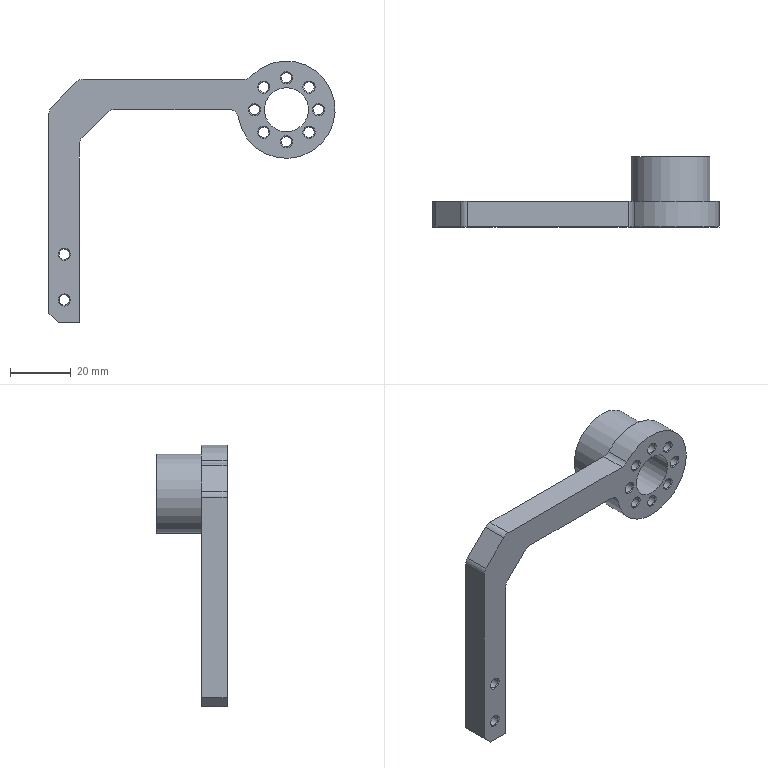Part | NX | features DATUM_CSYS 12, SKETCH 11, SIMPLE HOLE 10, HOLE PACKAGE 9, EXTRACT_FACE 8, Instance Feature 7, BLEND 2, CHAMFER 2, CPROJ 1, DATUM_AXIS 1, EXTRUDE 1, LINKED_FACE 1, OFFSET_REGION 1, Pattern Feature 1, SWP104 1 | 1 solid | 52 faces | box 93.991 x 23.1 x 85.991 mm | volume 19432 mm3 | cylinder 20 | cone 20 | plane 12 | commonest cylinder face diameters 3.4 x10 6 x6 14.463 x1 25.981 x1 29.983 x1 31.983 x1
STEP:
#1=CARTESIAN_POINT('',(-13.5,-14.1,-21.731));
#2=VERTEX_POINT('',#1);
#3=CARTESIAN_POINT('',(-13.5,-14.1,-14.5));
#4=DIRECTION('',(0.,-1.,0.));
#5=DIRECTION('',(0.,0.,-1.));
#6=AXIS2_PLACEMENT_3D('',#3,#4,#5);
#7=CIRCLE('',#6,7.231);
#8=EDGE_CURVE('',#2,#2,#7,.T.);
#9=ORIENTED_EDGE('',*,*,#8,.T.);
#10=EDGE_LOOP('',(#9));
#11=FACE_BOUND('',#10,.T.);
#12=CARTESIAN_POINT('',(-13.5,9.,-21.731));
#13=VERTEX_POINT('',#12);
#14=CARTESIAN_POINT('',(-13.5,9.,-14.5));
#15=DIRECTION('',(0.,-1.,0.));
#16=DIRECTION('',(0.,0.,-1.));
#17=AXIS2_PLACEMENT_3D('',#14,#15,#16);
#18=CIRCLE('',#17,7.231);
#19=EDGE_CURVE('',#13,#13,#18,.T.);
#20=ORIENTED_EDGE('',*,*,#19,.F.);
#21=EDGE_LOOP('',(#20));
#22=FACE_BOUND('',#21,.T.);
#23=CARTESIAN_POINT('',(-13.5,-13.36,-14.5));
#24=DIRECTION('',(0.,-1.,0.));
#25=DIRECTION('',(0.,0.,-1.));
#26=AXIS2_PLACEMENT_3D('',#23,#24,#25);
#27=CYLINDRICAL_SURFACE('',#26,7.231);
#28=ADVANCED_FACE('',(#11,#22),#27,.F.);
#29=CARTESIAN_POINT('',(-86.5,-14.1,-79.));
#30=VERTEX_POINT('',#29);
#31=CARTESIAN_POINT('',(-86.5,-14.1,-77.));
#32=DIRECTION('',(0.,-1.,0.));
#33=DIRECTION('',(0.,0.,-1.));
#34=AXIS2_PLACEMENT_3D('',#31,#32,#33);
#35=CIRCLE('',#34,2.);
#36=EDGE_CURVE('',#30,#30,#35,.F.);
#37=ORIENTED_EDGE('',*,*,#36,.T.);
#38=EDGE_LOOP('',(#37));
#39=FACE_BOUND('',#38,.T.);
#40=CARTESIAN_POINT('',(-86.5,-14.1,-64.));
#41=VERTEX_POINT('',#40);
#42=CARTESIAN_POINT('',(-86.5,-14.1,-62.));
#43=DIRECTION('',(0.,-1.,0.));
#44=DIRECTION('',(0.,0.,-1.));
#45=AXIS2_PLACEMENT_3D('',#42,#43,#44);
#46=CIRCLE('',#45,2.);
#47=EDGE_CURVE('',#41,#41,#46,.F.);
#48=ORIENTED_EDGE('',*,*,#47,.T.);
#49=EDGE_LOOP('',(#48));
#50=FACE_BOUND('',#49,.T.);
#51=CARTESIAN_POINT('',(-6.075,-14.1,-9.075));
#52=VERTEX_POINT('',#51);
#53=CARTESIAN_POINT('',(-6.075,-14.1,-7.075));
#54=DIRECTION('',(0.,-1.,0.));
#55=DIRECTION('',(0.,0.,-1.));
#56=AXIS2_PLACEMENT_3D('',#53,#54,#55);
#57=CIRCLE('',#56,2.);
#58=EDGE_CURVE('',#52,#52,#57,.F.);
#59=ORIENTED_EDGE('',*,*,#58,.T.);
#60=EDGE_LOOP('',(#59));
#61=FACE_BOUND('',#60,.T.);
#62=CARTESIAN_POINT('',(-3.,-14.1,-16.5));
#63=VERTEX_POINT('',#62);
#64=CARTESIAN_POINT('',(-3.,-14.1,-14.5));
#65=DIRECTION('',(0.,-1.,0.));
#66=DIRECTION('',(0.,0.,-1.));
#67=AXIS2_PLACEMENT_3D('',#64,#65,#66);
#68=CIRCLE('',#67,2.);
#69=EDGE_CURVE('',#63,#63,#68,.F.);
#70=ORIENTED_EDGE('',*,*,#69,.T.);
#71=EDGE_LOOP('',(#70));
#72=FACE_BOUND('',#71,.T.);
#73=CARTESIAN_POINT('',(-6.075,-14.1,-23.925));
#74=VERTEX_POINT('',#73);
#75=CARTESIAN_POINT('',(-6.075,-14.1,-21.925));
#76=DIRECTION('',(0.,-1.,0.));
#77=DIRECTION('',(0.,0.,-1.));
#78=AXIS2_PLACEMENT_3D('',#75,#76,#77);
#79=CIRCLE('',#78,2.);
#80=EDGE_CURVE('',#74,#74,#79,.F.);
#81=ORIENTED_EDGE('',*,*,#80,.T.);
#82=EDGE_LOOP('',(#81));
#83=FACE_BOUND('',#82,.T.);
#84=CARTESIAN_POINT('',(-13.5,-14.1,-27.));
#85=VERTEX_POINT('',#84);
#86=CARTESIAN_POINT('',(-13.5,-14.1,-25.));
#87=DIRECTION('',(0.,-1.,0.));
#88=DIRECTION('',(0.,0.,-1.));
#89=AXIS2_PLACEMENT_3D('',#86,#87,#88);
#90=CIRCLE('',#89,2.);
#91=EDGE_CURVE('',#85,#85,#90,.F.);
#92=ORIENTED_EDGE('',*,*,#91,.T.);
#93=EDGE_LOOP('',(#92));
#94=FACE_BOUND('',#93,.T.);
#95=CARTESIAN_POINT('',(-20.925,-14.1,-23.925));
#96=VERTEX_POINT('',#95);
#97=CARTESIAN_POINT('',(-20.925,-14.1,-21.925));
#98=DIRECTION('',(0.,-1.,0.));
#99=DIRECTION('',(0.,0.,-1.));
#100=AXIS2_PLACEMENT_3D('',#97,#98,#99);
#101=CIRCLE('',#100,2.);
#102=EDGE_CURVE('',#96,#96,#101,.F.);
#103=ORIENTED_EDGE('',*,*,#102,.T.);
#104=EDGE_LOOP('',(#103));
#105=FACE_BOUND('',#104,.T.);
#106=CARTESIAN_POINT('',(-24.,-14.1,-16.5));
#107=VERTEX_POINT('',#106);
#108=CARTESIAN_POINT('',(-24.,-14.1,-14.5));
#109=DIRECTION('',(0.,-1.,0.));
#110=DIRECTION('',(0.,0.,-1.));
#111=AXIS2_PLACEMENT_3D('',#108,#109,#110);
#112=CIRCLE('',#111,2.);
#113=EDGE_CURVE('',#107,#107,#112,.F.);
#114=ORIENTED_EDGE('',*,*,#113,.T.);
#115=EDGE_LOOP('',(#114));
#116=FACE_BOUND('',#115,.T.);
#117=CARTESIAN_POINT('',(-20.925,-14.1,-9.075));
#118=VERTEX_POINT('',#117);
#119=CARTESIAN_POINT('',(-20.925,-14.1,-7.075));
#120=DIRECTION('',(0.,-1.,0.));
#121=DIRECTION('',(0.,0.,-1.));
#122=AXIS2_PLACEMENT_3D('',#119,#120,#121);
#123=CIRCLE('',#122,2.);
#124=EDGE_CURVE('',#118,#118,#123,.F.);
#125=ORIENTED_EDGE('',*,*,#124,.T.);
#126=EDGE_LOOP('',(#125));
#127=FACE_BOUND('',#126,.T.);
#128=CARTESIAN_POINT('',(-13.5,-14.1,-6.));
#129=VERTEX_POINT('',#128);
#130=CARTESIAN_POINT('',(-13.5,-14.1,-4.));
#131=DIRECTION('',(0.,-1.,0.));
#132=DIRECTION('',(0.,0.,-1.));
#133=AXIS2_PLACEMENT_3D('',#130,#131,#132);
#134=CIRCLE('',#133,2.);
#135=EDGE_CURVE('',#129,#129,#134,.F.);
#136=ORIENTED_EDGE('',*,*,#135,.T.);
#137=EDGE_LOOP('',(#136));
#138=FACE_BOUND('',#137,.T.);
#139=CARTESIAN_POINT('',(-91.5,-14.1,-15.743));
#140=VERTEX_POINT('',#139);
#141=CARTESIAN_POINT('',(-91.5,-14.1,-81.5));
#142=VERTEX_POINT('',#141);
#143=CARTESIAN_POINT('',(-91.5,-14.1,-4.5));
#144=DIRECTION('',(0.,0.,-1.));
#145=VECTOR('',#144,1000.);
#146=LINE('',#143,#145);
#147=EDGE_CURVE('',#140,#142,#146,.T.);
#148=ORIENTED_EDGE('',*,*,#147,.T.);
#149=CARTESIAN_POINT('',(-88.5,-14.1,-84.5));
#150=VERTEX_POINT('',#149);
#151=CARTESIAN_POINT('',(-82.384,-14.1,-90.616));
#152=DIRECTION('',(-0.7071,0.,0.7071));
#153=VECTOR('',#152,1000.);
#154=LINE('',#151,#153);
#155=EDGE_CURVE('',#142,#150,#154,.F.);
#156=ORIENTED_EDGE('',*,*,#155,.T.);
#157=CARTESIAN_POINT('',(-81.5,-14.1,-84.5));
#158=VERTEX_POINT('',#157);
#159=CARTESIAN_POINT('',(-91.5,-14.1,-84.5));
#160=DIRECTION('',(1.,0.,0.));
#161=VECTOR('',#160,1000.);
#162=LINE('',#159,#161);
#163=EDGE_CURVE('',#150,#158,#162,.T.);
#164=ORIENTED_EDGE('',*,*,#163,.T.);
#165=CARTESIAN_POINT('',(-81.5,-14.1,-25.743));
#166=VERTEX_POINT('',#165);
#167=CARTESIAN_POINT('',(-81.5,-14.1,-84.5));
#168=DIRECTION('',(0.,0.,1.));
#169=VECTOR('',#168,1000.);
#170=LINE('',#167,#169);
#171=EDGE_CURVE('',#158,#166,#170,.T.);
#172=ORIENTED_EDGE('',*,*,#171,.T.);
#173=CARTESIAN_POINT('',(-80.621,-14.1,-23.621));
#174=VERTEX_POINT('',#173);
#175=CARTESIAN_POINT('',(-78.5,-14.1,-25.743));
#176=DIRECTION('',(0.,-1.,0.));
#177=DIRECTION('',(0.,0.,-1.));
#178=AXIS2_PLACEMENT_3D('',#175,#176,#177);
#179=CIRCLE('',#178,3.);
#180=EDGE_CURVE('',#166,#174,#179,.F.);
#181=ORIENTED_EDGE('',*,*,#180,.T.);
#182=CARTESIAN_POINT('',(-72.379,-14.1,-15.379));
#183=VERTEX_POINT('',#182);
#184=CARTESIAN_POINT('',(-81.5,-14.1,-24.5));
#185=DIRECTION('',(-0.7071,0.,-0.7071));
#186=VECTOR('',#185,1000.);
#187=LINE('',#184,#186);
#188=EDGE_CURVE('',#174,#183,#187,.F.);
#189=ORIENTED_EDGE('',*,*,#188,.T.);
#190=CARTESIAN_POINT('',(-70.257,-14.1,-14.5));
#191=VERTEX_POINT('',#190);
#192=CARTESIAN_POINT('',(-70.257,-14.1,-17.5));
#193=DIRECTION('',(0.,-1.,0.));
#194=DIRECTION('',(0.,0.,-1.));
#195=AXIS2_PLACEMENT_3D('',#192,#193,#194);
#196=CIRCLE('',#195,3.);
#197=EDGE_CURVE('',#183,#191,#196,.F.);
#198=ORIENTED_EDGE('',*,*,#197,.T.);
#199=CARTESIAN_POINT('',(-32.253,-14.1,-14.5));
#200=VERTEX_POINT('',#199);
#201=CARTESIAN_POINT('',(-81.5,-14.1,-14.5));
#202=DIRECTION('',(1.,0.,0.));
#203=VECTOR('',#202,1000.);
#204=LINE('',#201,#203);
#205=EDGE_CURVE('',#191,#200,#204,.T.);
#206=ORIENTED_EDGE('',*,*,#205,.T.);
#207=CARTESIAN_POINT('',(-29.291,-14.1,-17.026));
#208=VERTEX_POINT('',#207);
#209=CARTESIAN_POINT('',(-32.253,-14.1,-17.5));
#210=DIRECTION('',(0.,-1.,0.));
#211=DIRECTION('',(0.,0.,-1.));
#212=AXIS2_PLACEMENT_3D('',#209,#210,#211);
#213=CIRCLE('',#212,3.);
#214=EDGE_CURVE('',#200,#208,#213,.F.);
#215=ORIENTED_EDGE('',*,*,#214,.T.);
#216=CARTESIAN_POINT('',(-25.158,-14.1,-3.554));
#217=VERTEX_POINT('',#216);
#218=CARTESIAN_POINT('',(-13.5,-14.1,-14.5));
#219=DIRECTION('',(0.,-1.,0.));
#220=DIRECTION('',(0.,0.,-1.));
#221=AXIS2_PLACEMENT_3D('',#218,#219,#220);
#222=CIRCLE('',#221,15.991);
#223=EDGE_CURVE('',#208,#217,#222,.T.);
#224=ORIENTED_EDGE('',*,*,#223,.T.);
#225=CARTESIAN_POINT('',(-27.345,-14.1,-4.5));
#226=VERTEX_POINT('',#225);
#227=CARTESIAN_POINT('',(-27.345,-14.1,-1.5));
#228=DIRECTION('',(0.,-1.,0.));
#229=DIRECTION('',(0.,0.,-1.));
#230=AXIS2_PLACEMENT_3D('',#227,#228,#229);
#231=CIRCLE('',#230,3.);
#232=EDGE_CURVE('',#217,#226,#231,.F.);
#233=ORIENTED_EDGE('',*,*,#232,.T.);
#234=CARTESIAN_POINT('',(-80.257,-14.1,-4.5));
#235=VERTEX_POINT('',#234);
#236=CARTESIAN_POINT('',(-81.5,-14.1,-4.5));
#237=DIRECTION('',(-1.,0.,0.));
#238=VECTOR('',#237,1000.);
#239=LINE('',#236,#238);
#240=EDGE_CURVE('',#226,#235,#239,.T.);
#241=ORIENTED_EDGE('',*,*,#240,.T.);
#242=CARTESIAN_POINT('',(-82.379,-14.1,-5.379));
#243=VERTEX_POINT('',#242);
#244=CARTESIAN_POINT('',(-80.257,-14.1,-7.5));
#245=DIRECTION('',(0.,-1.,0.));
#246=DIRECTION('',(0.,0.,-1.));
#247=AXIS2_PLACEMENT_3D('',#244,#245,#246);
#248=CIRCLE('',#247,3.);
#249=EDGE_CURVE('',#235,#243,#248,.T.);
#250=ORIENTED_EDGE('',*,*,#249,.T.);
#251=CARTESIAN_POINT('',(-90.621,-14.1,-13.621));
#252=VERTEX_POINT('',#251);
#253=CARTESIAN_POINT('',(-48.884,-14.1,28.116));
#254=DIRECTION('',(0.7071,0.,0.7071));
#255=VECTOR('',#254,1000.);
#256=LINE('',#253,#255);
#257=EDGE_CURVE('',#243,#252,#256,.F.);
#258=ORIENTED_EDGE('',*,*,#257,.T.);
#259=CARTESIAN_POINT('',(-88.5,-14.1,-15.743));
#260=DIRECTION('',(0.,-1.,0.));
#261=DIRECTION('',(0.,0.,-1.));
#262=AXIS2_PLACEMENT_3D('',#259,#260,#261);
#263=CIRCLE('',#262,3.);
#264=EDGE_CURVE('',#252,#140,#263,.T.);
#265=ORIENTED_EDGE('',*,*,#264,.T.);
#266=EDGE_LOOP('',(#148,#156,#164,#172,#181,#189,#198,#206,#215,#224,#233,#241,#250,#258,#265));
#267=FACE_BOUND('',#266,.T.);
#268=ORIENTED_EDGE('',*,*,#8,.F.);
#269=EDGE_LOOP('',(#268));
#270=FACE_BOUND('',#269,.T.);
#271=CARTESIAN_POINT('',(-6.269,-14.1,-14.5));
#272=DIRECTION('',(0.,-1.,0.));
#273=DIRECTION('',(0.,0.,-1.));
#274=AXIS2_PLACEMENT_3D('',#271,#272,#273);
#275=PLANE('',#274);
#276=ADVANCED_FACE('',(#39,#50,#61,#72,#83,#94,#105,#116,#127,#138,#267,#270),#275,.T.);
#277=ORIENTED_EDGE('',*,*,#223,.F.);
#278=CARTESIAN_POINT('',(-29.291,-5.6,-17.026));
#279=VERTEX_POINT('',#278);
#280=CARTESIAN_POINT('',(-29.291,-13.36,-17.026));
#281=DIRECTION('',(0.,-1.,0.));
#282=VECTOR('',#281,1000.);
#283=LINE('',#280,#282);
#284=EDGE_CURVE('',#208,#279,#283,.F.);
#285=ORIENTED_EDGE('',*,*,#284,.T.);
#286=CARTESIAN_POINT('',(-25.158,-5.6,-3.554));
#287=VERTEX_POINT('',#286);
#288=CARTESIAN_POINT('',(-13.5,-5.6,-14.5));
#289=DIRECTION('',(0.,-1.,0.));
#290=DIRECTION('',(0.,0.,-1.));
#291=AXIS2_PLACEMENT_3D('',#288,#289,#290);
#292=CIRCLE('',#291,15.991);
#293=EDGE_CURVE('',#279,#287,#292,.T.);
#294=ORIENTED_EDGE('',*,*,#293,.T.);
#295=CARTESIAN_POINT('',(-25.158,-13.36,-3.554));
#296=DIRECTION('',(0.,-1.,0.));
#297=VECTOR('',#296,1000.);
#298=LINE('',#295,#297);
#299=EDGE_CURVE('',#287,#217,#298,.T.);
#300=ORIENTED_EDGE('',*,*,#299,.T.);
#301=EDGE_LOOP('',(#277,#285,#294,#300));
#302=FACE_BOUND('',#301,.T.);
#303=CARTESIAN_POINT('',(-13.5,-13.36,-14.5));
#304=DIRECTION('',(0.,-1.,0.));
#305=DIRECTION('',(0.,0.,-1.));
#306=AXIS2_PLACEMENT_3D('',#303,#304,#305);
#307=CYLINDRICAL_SURFACE('',#306,15.991);
#308=ADVANCED_FACE('',(#302),#307,.T.);
#309=CARTESIAN_POINT('',(-86.5,-5.6,-75.));
#310=VERTEX_POINT('',#309);
#311=CARTESIAN_POINT('',(-86.5,-5.6,-77.));
#312=DIRECTION('',(0.,1.,0.));
#313=DIRECTION('',(0.,0.,1.));
#314=AXIS2_PLACEMENT_3D('',#311,#312,#313);
#315=CIRCLE('',#314,2.);
#316=EDGE_CURVE('',#310,#310,#315,.F.);
#317=ORIENTED_EDGE('',*,*,#316,.T.);
#318=EDGE_LOOP('',(#317));
#319=FACE_BOUND('',#318,.T.);
#320=CARTESIAN_POINT('',(-86.5,-5.6,-60.));
#321=VERTEX_POINT('',#320);
#322=CARTESIAN_POINT('',(-86.5,-5.6,-62.));
#323=DIRECTION('',(0.,1.,0.));
#324=DIRECTION('',(0.,0.,1.));
#325=AXIS2_PLACEMENT_3D('',#322,#323,#324);
#326=CIRCLE('',#325,2.);
#327=EDGE_CURVE('',#321,#321,#326,.F.);
#328=ORIENTED_EDGE('',*,*,#327,.T.);
#329=EDGE_LOOP('',(#328));
#330=FACE_BOUND('',#329,.T.);
#331=CARTESIAN_POINT('',(-13.5,-5.6,-29.491));
#332=VERTEX_POINT('',#331);
#333=CARTESIAN_POINT('',(-13.5,-5.6,-14.5));
#334=DIRECTION('',(0.,-1.,0.));
#335=DIRECTION('',(0.,0.,-1.));
#336=AXIS2_PLACEMENT_3D('',#333,#334,#335);
#337=CIRCLE('',#336,14.991);
#338=EDGE_CURVE('',#332,#332,#337,.T.);
#339=ORIENTED_EDGE('',*,*,#338,.T.);
#340=EDGE_LOOP('',(#339));
#341=FACE_BOUND('',#340,.T.);
#342=CARTESIAN_POINT('',(-88.5,-5.6,-84.5));
#343=VERTEX_POINT('',#342);
#344=CARTESIAN_POINT('',(-81.5,-5.6,-84.5));
#345=VERTEX_POINT('',#344);
#346=CARTESIAN_POINT('',(-91.5,-5.6,-84.5));
#347=DIRECTION('',(1.,0.,0.));
#348=VECTOR('',#347,1000.);
#349=LINE('',#346,#348);
#350=EDGE_CURVE('',#343,#345,#349,.T.);
#351=ORIENTED_EDGE('',*,*,#350,.F.);
#352=CARTESIAN_POINT('',(-91.5,-5.6,-81.5));
#353=VERTEX_POINT('',#352);
#354=CARTESIAN_POINT('',(-78.004,-5.6,-94.996));
#355=DIRECTION('',(0.7071,0.,-0.7071));
#356=VECTOR('',#355,1000.);
#357=LINE('',#354,#356);
#358=EDGE_CURVE('',#343,#353,#357,.F.);
#359=ORIENTED_EDGE('',*,*,#358,.T.);
#360=CARTESIAN_POINT('',(-91.5,-5.6,-15.743));
#361=VERTEX_POINT('',#360);
#362=CARTESIAN_POINT('',(-91.5,-5.6,-14.5));
#363=DIRECTION('',(0.,0.,-1.));
#364=VECTOR('',#363,1000.);
#365=LINE('',#362,#364);
#366=EDGE_CURVE('',#361,#353,#365,.T.);
#367=ORIENTED_EDGE('',*,*,#366,.F.);
#368=CARTESIAN_POINT('',(-90.621,-5.6,-13.621));
#369=VERTEX_POINT('',#368);
#370=CARTESIAN_POINT('',(-88.5,-5.6,-15.743));
#371=DIRECTION('',(0.,1.,0.));
#372=DIRECTION('',(0.,0.,1.));
#373=AXIS2_PLACEMENT_3D('',#370,#371,#372);
#374=CIRCLE('',#373,3.);
#375=EDGE_CURVE('',#361,#369,#374,.T.);
#376=ORIENTED_EDGE('',*,*,#375,.T.);
#377=CARTESIAN_POINT('',(-82.379,-5.6,-5.379));
#378=VERTEX_POINT('',#377);
#379=CARTESIAN_POINT('',(-44.504,-5.6,32.496));
#380=DIRECTION('',(-0.7071,0.,-0.7071));
#381=VECTOR('',#380,1000.);
#382=LINE('',#379,#381);
#383=EDGE_CURVE('',#369,#378,#382,.F.);
#384=ORIENTED_EDGE('',*,*,#383,.T.);
#385=CARTESIAN_POINT('',(-80.257,-5.6,-4.5));
#386=VERTEX_POINT('',#385);
#387=CARTESIAN_POINT('',(-80.257,-5.6,-7.5));
#388=DIRECTION('',(0.,1.,0.));
#389=DIRECTION('',(0.,0.,1.));
#390=AXIS2_PLACEMENT_3D('',#387,#388,#389);
#391=CIRCLE('',#390,3.);
#392=EDGE_CURVE('',#378,#386,#391,.T.);
#393=ORIENTED_EDGE('',*,*,#392,.T.);
#394=CARTESIAN_POINT('',(-27.345,-5.6,-4.5));
#395=VERTEX_POINT('',#394);
#396=CARTESIAN_POINT('',(-25.979,-5.6,-4.5));
#397=DIRECTION('',(-1.,0.,0.));
#398=VECTOR('',#397,1000.);
#399=LINE('',#396,#398);
#400=EDGE_CURVE('',#395,#386,#399,.T.);
#401=ORIENTED_EDGE('',*,*,#400,.F.);
#402=CARTESIAN_POINT('',(-27.345,-5.6,-1.5));
#403=DIRECTION('',(0.,1.,0.));
#404=DIRECTION('',(0.,0.,1.));
#405=AXIS2_PLACEMENT_3D('',#402,#403,#404);
#406=CIRCLE('',#405,3.);
#407=EDGE_CURVE('',#395,#287,#406,.F.);
#408=ORIENTED_EDGE('',*,*,#407,.T.);
#409=ORIENTED_EDGE('',*,*,#293,.F.);
#410=CARTESIAN_POINT('',(-32.253,-5.6,-14.5));
#411=VERTEX_POINT('',#410);
#412=CARTESIAN_POINT('',(-32.253,-5.6,-17.5));
#413=DIRECTION('',(0.,1.,0.));
#414=DIRECTION('',(0.,0.,1.));
#415=AXIS2_PLACEMENT_3D('',#412,#413,#414);
#416=CIRCLE('',#415,3.);
#417=EDGE_CURVE('',#279,#411,#416,.F.);
#418=ORIENTED_EDGE('',*,*,#417,.T.);
#419=CARTESIAN_POINT('',(-70.257,-5.6,-14.5));
#420=VERTEX_POINT('',#419);
#421=CARTESIAN_POINT('',(-81.5,-5.6,-14.5));
#422=DIRECTION('',(1.,0.,0.));
#423=VECTOR('',#422,1000.);
#424=LINE('',#421,#423);
#425=EDGE_CURVE('',#420,#411,#424,.T.);
#426=ORIENTED_EDGE('',*,*,#425,.F.);
#427=CARTESIAN_POINT('',(-72.379,-5.6,-15.379));
#428=VERTEX_POINT('',#427);
#429=CARTESIAN_POINT('',(-70.257,-5.6,-17.5));
#430=DIRECTION('',(0.,1.,0.));
#431=DIRECTION('',(0.,0.,1.));
#432=AXIS2_PLACEMENT_3D('',#429,#430,#431);
#433=CIRCLE('',#432,3.);
#434=EDGE_CURVE('',#420,#428,#433,.F.);
#435=ORIENTED_EDGE('',*,*,#434,.T.);
#436=CARTESIAN_POINT('',(-80.621,-5.6,-23.621));
#437=VERTEX_POINT('',#436);
#438=CARTESIAN_POINT('',(-81.5,-5.6,-24.5));
#439=DIRECTION('',(0.7071,0.,0.7071));
#440=VECTOR('',#439,1000.);
#441=LINE('',#438,#440);
#442=EDGE_CURVE('',#428,#437,#441,.F.);
#443=ORIENTED_EDGE('',*,*,#442,.T.);
#444=CARTESIAN_POINT('',(-81.5,-5.6,-25.743));
#445=VERTEX_POINT('',#444);
#446=CARTESIAN_POINT('',(-78.5,-5.6,-25.743));
#447=DIRECTION('',(0.,1.,0.));
#448=DIRECTION('',(0.,0.,1.));
#449=AXIS2_PLACEMENT_3D('',#446,#447,#448);
#450=CIRCLE('',#449,3.);
#451=EDGE_CURVE('',#437,#445,#450,.F.);
#452=ORIENTED_EDGE('',*,*,#451,.T.);
#453=CARTESIAN_POINT('',(-81.5,-5.6,-84.5));
#454=DIRECTION('',(0.,0.,1.));
#455=VECTOR('',#454,1000.);
#456=LINE('',#453,#455);
#457=EDGE_CURVE('',#345,#445,#456,.T.);
#458=ORIENTED_EDGE('',*,*,#457,.F.);
#459=EDGE_LOOP('',(#351,#359,#367,#376,#384,#393,#401,#408,#409,#418,#426,#435,#443,#452,#458));
#460=FACE_BOUND('',#459,.T.);
#461=CARTESIAN_POINT('',(2.491,-5.6,-14.5));
#462=DIRECTION('',(0.,1.,0.));
#463=DIRECTION('',(0.,0.,1.));
#464=AXIS2_PLACEMENT_3D('',#461,#462,#463);
#465=PLANE('',#464);
#466=ADVANCED_FACE('',(#319,#330,#341,#460),#465,.T.);
#467=CARTESIAN_POINT('',(-13.5,-10.1,0.4914));
#468=VERTEX_POINT('',#467);
#469=CARTESIAN_POINT('',(-13.5,-10.1,-14.5));
#470=DIRECTION('',(0.,1.,0.));
#471=DIRECTION('',(0.,0.,1.));
#472=AXIS2_PLACEMENT_3D('',#469,#470,#471);
#473=CIRCLE('',#472,14.991);
#474=EDGE_CURVE('',#468,#468,#473,.F.);
#475=ORIENTED_EDGE('',*,*,#474,.T.);
#476=EDGE_LOOP('',(#475));
#477=FACE_BOUND('',#476,.T.);
#478=ORIENTED_EDGE('',*,*,#338,.F.);
#479=EDGE_LOOP('',(#478));
#480=FACE_BOUND('',#479,.T.);
#481=CARTESIAN_POINT('',(-13.5,-13.36,-14.5));
#482=DIRECTION('',(0.,-1.,0.));
#483=DIRECTION('',(0.,0.,-1.));
#484=AXIS2_PLACEMENT_3D('',#481,#482,#483);
#485=CYLINDRICAL_SURFACE('',#484,14.991);
#486=ADVANCED_FACE('',(#477,#480),#485,.F.);
#487=CARTESIAN_POINT('',(-13.5,-10.1,-1.509));
#488=VERTEX_POINT('',#487);
#489=CARTESIAN_POINT('',(-13.5,-10.1,-14.5));
#490=DIRECTION('',(0.,1.,0.));
#491=DIRECTION('',(0.,0.,1.));
#492=AXIS2_PLACEMENT_3D('',#489,#490,#491);
#493=CIRCLE('',#492,12.991);
#494=EDGE_CURVE('',#488,#488,#493,.F.);
#495=ORIENTED_EDGE('',*,*,#494,.T.);
#496=EDGE_LOOP('',(#495));
#497=FACE_BOUND('',#496,.T.);
#498=ORIENTED_EDGE('',*,*,#474,.F.);
#499=EDGE_LOOP('',(#498));
#500=FACE_BOUND('',#499,.T.);
#501=CARTESIAN_POINT('',(1.491,-10.1,-14.5));
#502=DIRECTION('',(0.,1.,0.));
#503=DIRECTION('',(0.,0.,1.));
#504=AXIS2_PLACEMENT_3D('',#501,#502,#503);
#505=PLANE('',#504);
#506=ADVANCED_FACE('',(#497,#500),#505,.T.);
#507=CARTESIAN_POINT('',(-13.5,9.,-27.491));
#508=VERTEX_POINT('',#507);
#509=CARTESIAN_POINT('',(-13.5,9.,-14.5));
#510=DIRECTION('',(0.,-1.,0.));
#511=DIRECTION('',(0.,0.,-1.));
#512=AXIS2_PLACEMENT_3D('',#509,#510,#511);
#513=CIRCLE('',#512,12.991);
#514=EDGE_CURVE('',#508,#508,#513,.T.);
#515=ORIENTED_EDGE('',*,*,#514,.T.);
#516=EDGE_LOOP('',(#515));
#517=FACE_BOUND('',#516,.T.);
#518=ORIENTED_EDGE('',*,*,#494,.F.);
#519=EDGE_LOOP('',(#518));
#520=FACE_BOUND('',#519,.T.);
#521=CARTESIAN_POINT('',(-13.5,-13.36,-14.5));
#522=DIRECTION('',(0.,-1.,0.));
#523=DIRECTION('',(0.,0.,-1.));
#524=AXIS2_PLACEMENT_3D('',#521,#522,#523);
#525=CYLINDRICAL_SURFACE('',#524,12.991);
#526=ADVANCED_FACE('',(#517,#520),#525,.T.);
#527=CARTESIAN_POINT('',(-6.075,9.,-5.075));
#528=VERTEX_POINT('',#527);
#529=CARTESIAN_POINT('',(-6.075,9.,-7.075));
#530=DIRECTION('',(0.,1.,0.));
#531=DIRECTION('',(0.,0.,1.));
#532=AXIS2_PLACEMENT_3D('',#529,#530,#531);
#533=CIRCLE('',#532,2.);
#534=EDGE_CURVE('',#528,#528,#533,.F.);
#535=ORIENTED_EDGE('',*,*,#534,.T.);
#536=EDGE_LOOP('',(#535));
#537=FACE_BOUND('',#536,.T.);
#538=CARTESIAN_POINT('',(-3.,9.,-12.5));
#539=VERTEX_POINT('',#538);
#540=CARTESIAN_POINT('',(-3.,9.,-14.5));
#541=DIRECTION('',(0.,1.,0.));
#542=DIRECTION('',(0.,0.,1.));
#543=AXIS2_PLACEMENT_3D('',#540,#541,#542);
#544=CIRCLE('',#543,2.);
#545=EDGE_CURVE('',#539,#539,#544,.F.);
#546=ORIENTED_EDGE('',*,*,#545,.T.);
#547=EDGE_LOOP('',(#546));
#548=FACE_BOUND('',#547,.T.);
#549=CARTESIAN_POINT('',(-6.075,9.,-19.925));
#550=VERTEX_POINT('',#549);
#551=CARTESIAN_POINT('',(-6.075,9.,-21.925));
#552=DIRECTION('',(0.,1.,0.));
#553=DIRECTION('',(0.,0.,1.));
#554=AXIS2_PLACEMENT_3D('',#551,#552,#553);
#555=CIRCLE('',#554,2.);
#556=EDGE_CURVE('',#550,#550,#555,.F.);
#557=ORIENTED_EDGE('',*,*,#556,.T.);
#558=EDGE_LOOP('',(#557));
#559=FACE_BOUND('',#558,.T.);
#560=CARTESIAN_POINT('',(-13.5,9.,-23.));
#561=VERTEX_POINT('',#560);
#562=CARTESIAN_POINT('',(-13.5,9.,-25.));
#563=DIRECTION('',(0.,1.,0.));
#564=DIRECTION('',(0.,0.,1.));
#565=AXIS2_PLACEMENT_3D('',#562,#563,#564);
#566=CIRCLE('',#565,2.);
#567=EDGE_CURVE('',#561,#561,#566,.F.);
#568=ORIENTED_EDGE('',*,*,#567,.T.);
#569=EDGE_LOOP('',(#568));
#570=FACE_BOUND('',#569,.T.);
#571=CARTESIAN_POINT('',(-20.925,9.,-19.925));
#572=VERTEX_POINT('',#571);
#573=CARTESIAN_POINT('',(-20.925,9.,-21.925));
#574=DIRECTION('',(0.,1.,0.));
#575=DIRECTION('',(0.,0.,1.));
#576=AXIS2_PLACEMENT_3D('',#573,#574,#575);
#577=CIRCLE('',#576,2.);
#578=EDGE_CURVE('',#572,#572,#577,.F.);
#579=ORIENTED_EDGE('',*,*,#578,.T.);
#580=EDGE_LOOP('',(#579));
#581=FACE_BOUND('',#580,.T.);
#582=CARTESIAN_POINT('',(-24.,9.,-12.5));
#583=VERTEX_POINT('',#582);
#584=CARTESIAN_POINT('',(-24.,9.,-14.5));
#585=DIRECTION('',(0.,1.,0.));
#586=DIRECTION('',(0.,0.,1.));
#587=AXIS2_PLACEMENT_3D('',#584,#585,#586);
#588=CIRCLE('',#587,2.);
#589=EDGE_CURVE('',#583,#583,#588,.F.);
#590=ORIENTED_EDGE('',*,*,#589,.T.);
#591=EDGE_LOOP('',(#590));
#592=FACE_BOUND('',#591,.T.);
#593=CARTESIAN_POINT('',(-20.925,9.,-5.075));
#594=VERTEX_POINT('',#593);
#595=CARTESIAN_POINT('',(-20.925,9.,-7.075));
#596=DIRECTION('',(0.,1.,0.));
#597=DIRECTION('',(0.,0.,1.));
#598=AXIS2_PLACEMENT_3D('',#595,#596,#597);
#599=CIRCLE('',#598,2.);
#600=EDGE_CURVE('',#594,#594,#599,.F.);
#601=ORIENTED_EDGE('',*,*,#600,.T.);
#602=EDGE_LOOP('',(#601));
#603=FACE_BOUND('',#602,.T.);
#604=CARTESIAN_POINT('',(-13.5,9.,-2.));
#605=VERTEX_POINT('',#604);
#606=CARTESIAN_POINT('',(-13.5,9.,-4.));
#607=DIRECTION('',(0.,1.,0.));
#608=DIRECTION('',(0.,0.,1.));
#609=AXIS2_PLACEMENT_3D('',#606,#607,#608);
#610=CIRCLE('',#609,2.);
#611=EDGE_CURVE('',#605,#605,#610,.F.);
#612=ORIENTED_EDGE('',*,*,#611,.T.);
#613=EDGE_LOOP('',(#612));
#614=FACE_BOUND('',#613,.T.);
#615=ORIENTED_EDGE('',*,*,#19,.T.);
#616=EDGE_LOOP('',(#615));
#617=FACE_BOUND('',#616,.T.);
#618=ORIENTED_EDGE('',*,*,#514,.F.);
#619=EDGE_LOOP('',(#618));
#620=FACE_BOUND('',#619,.T.);
#621=CARTESIAN_POINT('',(-0.5093,9.,-14.5));
#622=DIRECTION('',(0.,1.,0.));
#623=DIRECTION('',(0.,0.,1.));
#624=AXIS2_PLACEMENT_3D('',#621,#622,#623);
#625=PLANE('',#624);
#626=ADVANCED_FACE('',(#537,#548,#559,#570,#581,#592,#603,#614,#617,#620),#625,.T.);
#627=ORIENTED_EDGE('',*,*,#163,.F.);
#628=CARTESIAN_POINT('',(-88.5,-5.6,-84.5));
#629=DIRECTION('',(0.,1.,0.));
#630=VECTOR('',#629,1000.);
#631=LINE('',#628,#630);
#632=EDGE_CURVE('',#150,#343,#631,.T.);
#633=ORIENTED_EDGE('',*,*,#632,.T.);
#634=ORIENTED_EDGE('',*,*,#350,.T.);
#635=CARTESIAN_POINT('',(-81.5,-5.6,-84.5));
#636=DIRECTION('',(0.,-1.,0.));
#637=VECTOR('',#636,1000.);
#638=LINE('',#635,#637);
#639=EDGE_CURVE('',#345,#158,#638,.T.);
#640=ORIENTED_EDGE('',*,*,#639,.T.);
#641=EDGE_LOOP('',(#627,#633,#634,#640));
#642=FACE_BOUND('',#641,.T.);
#643=CARTESIAN_POINT('',(-91.5,-5.6,-84.5));
#644=DIRECTION('',(0.,0.,-1.));
#645=DIRECTION('',(-1.,0.,0.));
#646=AXIS2_PLACEMENT_3D('',#643,#644,#645);
#647=PLANE('',#646);
#648=ADVANCED_FACE('',(#642),#647,.T.);
#649=ORIENTED_EDGE('',*,*,#457,.T.);
#650=CARTESIAN_POINT('',(-81.5,-5.6,-25.743));
#651=DIRECTION('',(0.,1.,0.));
#652=VECTOR('',#651,1000.);
#653=LINE('',#650,#652);
#654=EDGE_CURVE('',#445,#166,#653,.F.);
#655=ORIENTED_EDGE('',*,*,#654,.T.);
#656=ORIENTED_EDGE('',*,*,#171,.F.);
#657=ORIENTED_EDGE('',*,*,#639,.F.);
#658=EDGE_LOOP('',(#649,#655,#656,#657));
#659=FACE_BOUND('',#658,.T.);
#660=CARTESIAN_POINT('',(-81.5,-5.6,-84.5));
#661=DIRECTION('',(1.,0.,0.));
#662=DIRECTION('',(0.,0.,-1.));
#663=AXIS2_PLACEMENT_3D('',#660,#661,#662);
#664=PLANE('',#663);
#665=ADVANCED_FACE('',(#659),#664,.T.);
#666=ORIENTED_EDGE('',*,*,#425,.T.);
#667=CARTESIAN_POINT('',(-32.253,-14.1,-14.5));
#668=DIRECTION('',(0.,1.,0.));
#669=VECTOR('',#668,1000.);
#670=LINE('',#667,#669);
#671=EDGE_CURVE('',#411,#200,#670,.F.);
#672=ORIENTED_EDGE('',*,*,#671,.T.);
#673=ORIENTED_EDGE('',*,*,#205,.F.);
#674=CARTESIAN_POINT('',(-70.257,-5.6,-14.5));
#675=DIRECTION('',(0.,-1.,0.));
#676=VECTOR('',#675,1000.);
#677=LINE('',#674,#676);
#678=EDGE_CURVE('',#191,#420,#677,.F.);
#679=ORIENTED_EDGE('',*,*,#678,.T.);
#680=EDGE_LOOP('',(#666,#672,#673,#679));
#681=FACE_BOUND('',#680,.T.);
#682=CARTESIAN_POINT('',(-81.5,-5.6,-14.5));
#683=DIRECTION('',(0.,0.,-1.));
#684=DIRECTION('',(-1.,0.,0.));
#685=AXIS2_PLACEMENT_3D('',#682,#683,#684);
#686=PLANE('',#685);
#687=ADVANCED_FACE('',(#681),#686,.T.);
#688=ORIENTED_EDGE('',*,*,#240,.F.);
#689=CARTESIAN_POINT('',(-27.345,-5.6,-4.5));
#690=DIRECTION('',(0.,1.,0.));
#691=VECTOR('',#690,1000.);
#692=LINE('',#689,#691);
#693=EDGE_CURVE('',#226,#395,#692,.T.);
#694=ORIENTED_EDGE('',*,*,#693,.T.);
#695=ORIENTED_EDGE('',*,*,#400,.T.);
#696=CARTESIAN_POINT('',(-80.257,-5.6,-4.5));
#697=DIRECTION('',(0.,1.,0.));
#698=VECTOR('',#697,1000.);
#699=LINE('',#696,#698);
#700=EDGE_CURVE('',#386,#235,#699,.F.);
#701=ORIENTED_EDGE('',*,*,#700,.T.);
#702=EDGE_LOOP('',(#688,#694,#695,#701));
#703=FACE_BOUND('',#702,.T.);
#704=CARTESIAN_POINT('',(-81.5,-5.6,-4.5));
#705=DIRECTION('',(0.,0.,1.));
#706=DIRECTION('',(1.,0.,0.));
#707=AXIS2_PLACEMENT_3D('',#704,#705,#706);
#708=PLANE('',#707);
#709=ADVANCED_FACE('',(#703),#708,.T.);
#710=ORIENTED_EDGE('',*,*,#366,.T.);
#711=CARTESIAN_POINT('',(-91.5,-5.6,-81.5));
#712=DIRECTION('',(0.,-1.,0.));
#713=VECTOR('',#712,1000.);
#714=LINE('',#711,#713);
#715=EDGE_CURVE('',#353,#142,#714,.T.);
#716=ORIENTED_EDGE('',*,*,#715,.T.);
#717=ORIENTED_EDGE('',*,*,#147,.F.);
#718=CARTESIAN_POINT('',(-91.5,-5.6,-15.743));
#719=DIRECTION('',(0.,-1.,0.));
#720=VECTOR('',#719,1000.);
#721=LINE('',#718,#720);
#722=EDGE_CURVE('',#140,#361,#721,.F.);
#723=ORIENTED_EDGE('',*,*,#722,.T.);
#724=EDGE_LOOP('',(#710,#716,#717,#723));
#725=FACE_BOUND('',#724,.T.);
#726=CARTESIAN_POINT('',(-91.5,-5.6,-4.5));
#727=DIRECTION('',(-1.,0.,0.));
#728=DIRECTION('',(0.,0.,1.));
#729=AXIS2_PLACEMENT_3D('',#726,#727,#728);
#730=PLANE('',#729);
#731=ADVANCED_FACE('',(#725),#730,.T.);
#732=ORIENTED_EDGE('',*,*,#383,.F.);
#733=CARTESIAN_POINT('',(-90.621,-5.6,-13.621));
#734=DIRECTION('',(0.,1.,0.));
#735=VECTOR('',#734,1000.);
#736=LINE('',#733,#735);
#737=EDGE_CURVE('',#369,#252,#736,.F.);
#738=ORIENTED_EDGE('',*,*,#737,.T.);
#739=ORIENTED_EDGE('',*,*,#257,.F.);
#740=CARTESIAN_POINT('',(-82.379,-5.6,-5.379));
#741=DIRECTION('',(0.,-1.,0.));
#742=VECTOR('',#741,1000.);
#743=LINE('',#740,#742);
#744=EDGE_CURVE('',#243,#378,#743,.F.);
#745=ORIENTED_EDGE('',*,*,#744,.T.);
#746=EDGE_LOOP('',(#732,#738,#739,#745));
#747=FACE_BOUND('',#746,.T.);
#748=CARTESIAN_POINT('',(-81.5,-5.6,-4.5));
#749=DIRECTION('',(0.7071,0.,-0.7071));
#750=DIRECTION('',(0.,-1.,0.));
#751=AXIS2_PLACEMENT_3D('',#748,#749,#750);
#752=PLANE('',#751);
#753=ADVANCED_FACE('',(#747),#752,.F.);
#754=ORIENTED_EDGE('',*,*,#188,.F.);
#755=CARTESIAN_POINT('',(-80.621,-5.6,-23.621));
#756=DIRECTION('',(0.,-1.,0.));
#757=VECTOR('',#756,1000.);
#758=LINE('',#755,#757);
#759=EDGE_CURVE('',#174,#437,#758,.F.);
#760=ORIENTED_EDGE('',*,*,#759,.T.);
#761=ORIENTED_EDGE('',*,*,#442,.F.);
#762=CARTESIAN_POINT('',(-72.379,-5.6,-15.379));
#763=DIRECTION('',(0.,1.,0.));
#764=VECTOR('',#763,1000.);
#765=LINE('',#762,#764);
#766=EDGE_CURVE('',#428,#183,#765,.F.);
#767=ORIENTED_EDGE('',*,*,#766,.T.);
#768=EDGE_LOOP('',(#754,#760,#761,#767));
#769=FACE_BOUND('',#768,.T.);
#770=CARTESIAN_POINT('',(-81.5,-5.6,-24.5));
#771=DIRECTION('',(0.7071,0.,-0.7071));
#772=DIRECTION('',(0.,1.,0.));
#773=AXIS2_PLACEMENT_3D('',#770,#771,#772);
#774=PLANE('',#773);
#775=ADVANCED_FACE('',(#769),#774,.T.);
#776=ORIENTED_EDGE('',*,*,#451,.F.);
#777=ORIENTED_EDGE('',*,*,#759,.F.);
#778=ORIENTED_EDGE('',*,*,#180,.F.);
#779=ORIENTED_EDGE('',*,*,#654,.F.);
#780=EDGE_LOOP('',(#776,#777,#778,#779));
#781=FACE_BOUND('',#780,.T.);
#782=CARTESIAN_POINT('',(-78.5,-5.6,-25.743));
#783=DIRECTION('',(0.,1.,0.));
#784=DIRECTION('',(0.,0.,1.));
#785=AXIS2_PLACEMENT_3D('',#782,#783,#784);
#786=CYLINDRICAL_SURFACE('',#785,3.);
#787=ADVANCED_FACE('',(#781),#786,.F.);
#788=ORIENTED_EDGE('',*,*,#197,.F.);
#789=ORIENTED_EDGE('',*,*,#766,.F.);
#790=ORIENTED_EDGE('',*,*,#434,.F.);
#791=ORIENTED_EDGE('',*,*,#678,.F.);
#792=EDGE_LOOP('',(#788,#789,#790,#791));
#793=FACE_BOUND('',#792,.T.);
#794=CARTESIAN_POINT('',(-70.257,-5.6,-17.5));
#795=DIRECTION('',(0.,-1.,0.));
#796=DIRECTION('',(0.,0.,-1.));
#797=AXIS2_PLACEMENT_3D('',#794,#795,#796);
#798=CYLINDRICAL_SURFACE('',#797,3.);
#799=ADVANCED_FACE('',(#793),#798,.F.);
#800=ORIENTED_EDGE('',*,*,#264,.F.);
#801=ORIENTED_EDGE('',*,*,#737,.F.);
#802=ORIENTED_EDGE('',*,*,#375,.F.);
#803=ORIENTED_EDGE('',*,*,#722,.F.);
#804=EDGE_LOOP('',(#800,#801,#802,#803));
#805=FACE_BOUND('',#804,.T.);
#806=CARTESIAN_POINT('',(-88.5,-5.6,-15.743));
#807=DIRECTION('',(0.,-1.,0.));
#808=DIRECTION('',(0.,0.,-1.));
#809=AXIS2_PLACEMENT_3D('',#806,#807,#808);
#810=CYLINDRICAL_SURFACE('',#809,3.);
#811=ADVANCED_FACE('',(#805),#810,.T.);
#812=ORIENTED_EDGE('',*,*,#392,.F.);
#813=ORIENTED_EDGE('',*,*,#744,.F.);
#814=ORIENTED_EDGE('',*,*,#249,.F.);
#815=ORIENTED_EDGE('',*,*,#700,.F.);
#816=EDGE_LOOP('',(#812,#813,#814,#815));
#817=FACE_BOUND('',#816,.T.);
#818=CARTESIAN_POINT('',(-80.257,-5.6,-7.5));
#819=DIRECTION('',(0.,1.,0.));
#820=DIRECTION('',(0.,0.,1.));
#821=AXIS2_PLACEMENT_3D('',#818,#819,#820);
#822=CYLINDRICAL_SURFACE('',#821,3.);
#823=ADVANCED_FACE('',(#817),#822,.T.);
#824=ORIENTED_EDGE('',*,*,#358,.F.);
#825=ORIENTED_EDGE('',*,*,#632,.F.);
#826=ORIENTED_EDGE('',*,*,#155,.F.);
#827=ORIENTED_EDGE('',*,*,#715,.F.);
#828=EDGE_LOOP('',(#824,#825,#826,#827));
#829=FACE_BOUND('',#828,.T.);
#830=CARTESIAN_POINT('',(-91.5,-5.6,-81.5));
#831=DIRECTION('',(0.7071,0.,0.7071));
#832=DIRECTION('',(0.,-1.,0.));
#833=AXIS2_PLACEMENT_3D('',#830,#831,#832);
#834=PLANE('',#833);
#835=ADVANCED_FACE('',(#829),#834,.F.);
#836=CARTESIAN_POINT('',(-13.5,8.7,-2.3));
#837=VERTEX_POINT('',#836);
#838=CARTESIAN_POINT('',(-13.5,8.7,-4.));
#839=DIRECTION('',(0.,1.,0.));
#840=DIRECTION('',(0.,0.,1.));
#841=AXIS2_PLACEMENT_3D('',#838,#839,#840);
#842=CIRCLE('',#841,1.7);
#843=EDGE_CURVE('',#837,#837,#842,.T.);
#844=ORIENTED_EDGE('',*,*,#843,.T.);
#845=EDGE_LOOP('',(#844));
#846=FACE_BOUND('',#845,.T.);
#847=CARTESIAN_POINT('',(-13.5,-13.8,-5.7));
#848=VERTEX_POINT('',#847);
#849=CARTESIAN_POINT('',(-13.5,-13.8,-4.));
#850=DIRECTION('',(0.,-1.,0.));
#851=DIRECTION('',(0.,0.,-1.));
#852=AXIS2_PLACEMENT_3D('',#849,#850,#851);
#853=CIRCLE('',#852,1.7);
#854=EDGE_CURVE('',#848,#848,#853,.T.);
#855=ORIENTED_EDGE('',*,*,#854,.T.);
#856=EDGE_LOOP('',(#855));
#857=FACE_BOUND('',#856,.T.);
#858=CARTESIAN_POINT('',(-13.5,-14.1,-4.));
#859=DIRECTION('',(0.,1.,0.));
#860=DIRECTION('',(0.,0.,1.));
#861=AXIS2_PLACEMENT_3D('',#858,#859,#860);
#862=CYLINDRICAL_SURFACE('',#861,1.7);
#863=ADVANCED_FACE('',(#846,#857),#862,.F.);
#864=ORIENTED_EDGE('',*,*,#854,.F.);
#865=EDGE_LOOP('',(#864));
#866=FACE_BOUND('',#865,.T.);
#867=ORIENTED_EDGE('',*,*,#135,.F.);
#868=EDGE_LOOP('',(#867));
#869=FACE_BOUND('',#868,.T.);
#870=CARTESIAN_POINT('',(-13.5,-14.1,-4.));
#871=DIRECTION('',(0.,-1.,0.));
#872=DIRECTION('',(0.,0.,-1.));
#873=AXIS2_PLACEMENT_3D('',#870,#871,#872);
#874=CONICAL_SURFACE('',#873,2.,0.7854);
#875=ADVANCED_FACE('',(#866,#869),#874,.F.);
#876=ORIENTED_EDGE('',*,*,#611,.F.);
#877=EDGE_LOOP('',(#876));
#878=FACE_BOUND('',#877,.T.);
#879=ORIENTED_EDGE('',*,*,#843,.F.);
#880=EDGE_LOOP('',(#879));
#881=FACE_BOUND('',#880,.T.);
#882=CARTESIAN_POINT('',(-13.5,8.7,-4.));
#883=DIRECTION('',(0.,1.,0.));
#884=DIRECTION('',(0.,0.,1.));
#885=AXIS2_PLACEMENT_3D('',#882,#883,#884);
#886=CONICAL_SURFACE('',#885,1.7,0.7854);
#887=ADVANCED_FACE('',(#878,#881),#886,.F.);
#888=CARTESIAN_POINT('',(-20.925,8.7,-5.375));
#889=VERTEX_POINT('',#888);
#890=CARTESIAN_POINT('',(-20.925,8.7,-7.075));
#891=DIRECTION('',(0.,1.,0.));
#892=DIRECTION('',(0.,0.,1.));
#893=AXIS2_PLACEMENT_3D('',#890,#891,#892);
#894=CIRCLE('',#893,1.7);
#895=EDGE_CURVE('',#889,#889,#894,.T.);
#896=ORIENTED_EDGE('',*,*,#895,.T.);
#897=EDGE_LOOP('',(#896));
#898=FACE_BOUND('',#897,.T.);
#899=CARTESIAN_POINT('',(-20.925,-13.8,-8.775));
#900=VERTEX_POINT('',#899);
#901=CARTESIAN_POINT('',(-20.925,-13.8,-7.075));
#902=DIRECTION('',(0.,-1.,0.));
#903=DIRECTION('',(0.,0.,-1.));
#904=AXIS2_PLACEMENT_3D('',#901,#902,#903);
#905=CIRCLE('',#904,1.7);
#906=EDGE_CURVE('',#900,#900,#905,.T.);
#907=ORIENTED_EDGE('',*,*,#906,.T.);
#908=EDGE_LOOP('',(#907));
#909=FACE_BOUND('',#908,.T.);
#910=CARTESIAN_POINT('',(-20.925,-14.1,-7.075));
#911=DIRECTION('',(0.,1.,0.));
#912=DIRECTION('',(0.,0.,1.));
#913=AXIS2_PLACEMENT_3D('',#910,#911,#912);
#914=CYLINDRICAL_SURFACE('',#913,1.7);
#915=ADVANCED_FACE('',(#898,#909),#914,.F.);
#916=ORIENTED_EDGE('',*,*,#906,.F.);
#917=EDGE_LOOP('',(#916));
#918=FACE_BOUND('',#917,.T.);
#919=ORIENTED_EDGE('',*,*,#124,.F.);
#920=EDGE_LOOP('',(#919));
#921=FACE_BOUND('',#920,.T.);
#922=CARTESIAN_POINT('',(-20.925,-14.1,-7.075));
#923=DIRECTION('',(0.,-1.,0.));
#924=DIRECTION('',(0.,0.,-1.));
#925=AXIS2_PLACEMENT_3D('',#922,#923,#924);
#926=CONICAL_SURFACE('',#925,2.,0.7854);
#927=ADVANCED_FACE('',(#918,#921),#926,.F.);
#928=ORIENTED_EDGE('',*,*,#600,.F.);
#929=EDGE_LOOP('',(#928));
#930=FACE_BOUND('',#929,.T.);
#931=ORIENTED_EDGE('',*,*,#895,.F.);
#932=EDGE_LOOP('',(#931));
#933=FACE_BOUND('',#932,.T.);
#934=CARTESIAN_POINT('',(-20.925,8.7,-7.075));
#935=DIRECTION('',(0.,1.,0.));
#936=DIRECTION('',(0.,0.,1.));
#937=AXIS2_PLACEMENT_3D('',#934,#935,#936);
#938=CONICAL_SURFACE('',#937,1.7,0.7854);
#939=ADVANCED_FACE('',(#930,#933),#938,.F.);
#940=CARTESIAN_POINT('',(-24.,8.7,-12.8));
#941=VERTEX_POINT('',#940);
#942=CARTESIAN_POINT('',(-24.,8.7,-14.5));
#943=DIRECTION('',(0.,1.,0.));
#944=DIRECTION('',(0.,0.,1.));
#945=AXIS2_PLACEMENT_3D('',#942,#943,#944);
#946=CIRCLE('',#945,1.7);
#947=EDGE_CURVE('',#941,#941,#946,.T.);
#948=ORIENTED_EDGE('',*,*,#947,.T.);
#949=EDGE_LOOP('',(#948));
#950=FACE_BOUND('',#949,.T.);
#951=CARTESIAN_POINT('',(-24.,-13.8,-16.2));
#952=VERTEX_POINT('',#951);
#953=CARTESIAN_POINT('',(-24.,-13.8,-14.5));
#954=DIRECTION('',(0.,-1.,0.));
#955=DIRECTION('',(0.,0.,-1.));
#956=AXIS2_PLACEMENT_3D('',#953,#954,#955);
#957=CIRCLE('',#956,1.7);
#958=EDGE_CURVE('',#952,#952,#957,.T.);
#959=ORIENTED_EDGE('',*,*,#958,.T.);
#960=EDGE_LOOP('',(#959));
#961=FACE_BOUND('',#960,.T.);
#962=CARTESIAN_POINT('',(-24.,-14.1,-14.5));
#963=DIRECTION('',(0.,1.,0.));
#964=DIRECTION('',(0.,0.,1.));
#965=AXIS2_PLACEMENT_3D('',#962,#963,#964);
#966=CYLINDRICAL_SURFACE('',#965,1.7);
#967=ADVANCED_FACE('',(#950,#961),#966,.F.);
#968=ORIENTED_EDGE('',*,*,#958,.F.);
#969=EDGE_LOOP('',(#968));
#970=FACE_BOUND('',#969,.T.);
#971=ORIENTED_EDGE('',*,*,#113,.F.);
#972=EDGE_LOOP('',(#971));
#973=FACE_BOUND('',#972,.T.);
#974=CARTESIAN_POINT('',(-24.,-14.1,-14.5));
#975=DIRECTION('',(0.,-1.,0.));
#976=DIRECTION('',(0.,0.,-1.));
#977=AXIS2_PLACEMENT_3D('',#974,#975,#976);
#978=CONICAL_SURFACE('',#977,2.,0.7854);
#979=ADVANCED_FACE('',(#970,#973),#978,.F.);
#980=ORIENTED_EDGE('',*,*,#589,.F.);
#981=EDGE_LOOP('',(#980));
#982=FACE_BOUND('',#981,.T.);
#983=ORIENTED_EDGE('',*,*,#947,.F.);
#984=EDGE_LOOP('',(#983));
#985=FACE_BOUND('',#984,.T.);
#986=CARTESIAN_POINT('',(-24.,8.7,-14.5));
#987=DIRECTION('',(0.,1.,0.));
#988=DIRECTION('',(0.,0.,1.));
#989=AXIS2_PLACEMENT_3D('',#986,#987,#988);
#990=CONICAL_SURFACE('',#989,1.7,0.7854);
#991=ADVANCED_FACE('',(#982,#985),#990,.F.);
#992=CARTESIAN_POINT('',(-20.925,8.7,-20.225));
#993=VERTEX_POINT('',#992);
#994=CARTESIAN_POINT('',(-20.925,8.7,-21.925));
#995=DIRECTION('',(0.,1.,0.));
#996=DIRECTION('',(0.,0.,1.));
#997=AXIS2_PLACEMENT_3D('',#994,#995,#996);
#998=CIRCLE('',#997,1.7);
#999=EDGE_CURVE('',#993,#993,#998,.T.);
#1000=ORIENTED_EDGE('',*,*,#999,.T.);
#1001=EDGE_LOOP('',(#1000));
#1002=FACE_BOUND('',#1001,.T.);
#1003=CARTESIAN_POINT('',(-20.925,-13.8,-23.625));
#1004=VERTEX_POINT('',#1003);
#1005=CARTESIAN_POINT('',(-20.925,-13.8,-21.925));
#1006=DIRECTION('',(0.,-1.,0.));
#1007=DIRECTION('',(0.,0.,-1.));
#1008=AXIS2_PLACEMENT_3D('',#1005,#1006,#1007);
#1009=CIRCLE('',#1008,1.7);
#1010=EDGE_CURVE('',#1004,#1004,#1009,.T.);
#1011=ORIENTED_EDGE('',*,*,#1010,.T.);
#1012=EDGE_LOOP('',(#1011));
#1013=FACE_BOUND('',#1012,.T.);
#1014=CARTESIAN_POINT('',(-20.925,-14.1,-21.925));
#1015=DIRECTION('',(0.,1.,0.));
#1016=DIRECTION('',(0.,0.,1.));
#1017=AXIS2_PLACEMENT_3D('',#1014,#1015,#1016);
#1018=CYLINDRICAL_SURFACE('',#1017,1.7);
#1019=ADVANCED_FACE('',(#1002,#1013),#1018,.F.);
#1020=ORIENTED_EDGE('',*,*,#1010,.F.);
#1021=EDGE_LOOP('',(#1020));
#1022=FACE_BOUND('',#1021,.T.);
#1023=ORIENTED_EDGE('',*,*,#102,.F.);
#1024=EDGE_LOOP('',(#1023));
#1025=FACE_BOUND('',#1024,.T.);
#1026=CARTESIAN_POINT('',(-20.925,-14.1,-21.925));
#1027=DIRECTION('',(0.,-1.,0.));
#1028=DIRECTION('',(0.,0.,-1.));
#1029=AXIS2_PLACEMENT_3D('',#1026,#1027,#1028);
#1030=CONICAL_SURFACE('',#1029,2.,0.7854);
#1031=ADVANCED_FACE('',(#1022,#1025),#1030,.F.);
#1032=ORIENTED_EDGE('',*,*,#578,.F.);
#1033=EDGE_LOOP('',(#1032));
#1034=FACE_BOUND('',#1033,.T.);
#1035=ORIENTED_EDGE('',*,*,#999,.F.);
#1036=EDGE_LOOP('',(#1035));
#1037=FACE_BOUND('',#1036,.T.);
#1038=CARTESIAN_POINT('',(-20.925,8.7,-21.925));
#1039=DIRECTION('',(0.,1.,0.));
#1040=DIRECTION('',(0.,0.,1.));
#1041=AXIS2_PLACEMENT_3D('',#1038,#1039,#1040);
#1042=CONICAL_SURFACE('',#1041,1.7,0.7854);
#1043=ADVANCED_FACE('',(#1034,#1037),#1042,.F.);
#1044=CARTESIAN_POINT('',(-13.5,8.7,-23.3));
#1045=VERTEX_POINT('',#1044);
#1046=CARTESIAN_POINT('',(-13.5,8.7,-25.));
#1047=DIRECTION('',(0.,1.,0.));
#1048=DIRECTION('',(0.,0.,1.));
#1049=AXIS2_PLACEMENT_3D('',#1046,#1047,#1048);
#1050=CIRCLE('',#1049,1.7);
#1051=EDGE_CURVE('',#1045,#1045,#1050,.T.);
#1052=ORIENTED_EDGE('',*,*,#1051,.T.);
#1053=EDGE_LOOP('',(#1052));
#1054=FACE_BOUND('',#1053,.T.);
#1055=CARTESIAN_POINT('',(-13.5,-13.8,-26.7));
#1056=VERTEX_POINT('',#1055);
#1057=CARTESIAN_POINT('',(-13.5,-13.8,-25.));
#1058=DIRECTION('',(0.,-1.,0.));
#1059=DIRECTION('',(0.,0.,-1.));
#1060=AXIS2_PLACEMENT_3D('',#1057,#1058,#1059);
#1061=CIRCLE('',#1060,1.7);
#1062=EDGE_CURVE('',#1056,#1056,#1061,.T.);
#1063=ORIENTED_EDGE('',*,*,#1062,.T.);
#1064=EDGE_LOOP('',(#1063));
#1065=FACE_BOUND('',#1064,.T.);
#1066=CARTESIAN_POINT('',(-13.5,-14.1,-25.));
#1067=DIRECTION('',(0.,1.,0.));
#1068=DIRECTION('',(0.,0.,1.));
#1069=AXIS2_PLACEMENT_3D('',#1066,#1067,#1068);
#1070=CYLINDRICAL_SURFACE('',#1069,1.7);
#1071=ADVANCED_FACE('',(#1054,#1065),#1070,.F.);
#1072=ORIENTED_EDGE('',*,*,#1062,.F.);
#1073=EDGE_LOOP('',(#1072));
#1074=FACE_BOUND('',#1073,.T.);
#1075=ORIENTED_EDGE('',*,*,#91,.F.);
#1076=EDGE_LOOP('',(#1075));
#1077=FACE_BOUND('',#1076,.T.);
#1078=CARTESIAN_POINT('',(-13.5,-14.1,-25.));
#1079=DIRECTION('',(0.,-1.,0.));
#1080=DIRECTION('',(0.,0.,-1.));
#1081=AXIS2_PLACEMENT_3D('',#1078,#1079,#1080);
#1082=CONICAL_SURFACE('',#1081,2.,0.7854);
#1083=ADVANCED_FACE('',(#1074,#1077),#1082,.F.);
#1084=ORIENTED_EDGE('',*,*,#567,.F.);
#1085=EDGE_LOOP('',(#1084));
#1086=FACE_BOUND('',#1085,.T.);
#1087=ORIENTED_EDGE('',*,*,#1051,.F.);
#1088=EDGE_LOOP('',(#1087));
#1089=FACE_BOUND('',#1088,.T.);
#1090=CARTESIAN_POINT('',(-13.5,8.7,-25.));
#1091=DIRECTION('',(0.,1.,0.));
#1092=DIRECTION('',(0.,0.,1.));
#1093=AXIS2_PLACEMENT_3D('',#1090,#1091,#1092);
#1094=CONICAL_SURFACE('',#1093,1.7,0.7854);
#1095=ADVANCED_FACE('',(#1086,#1089),#1094,.F.);
#1096=CARTESIAN_POINT('',(-6.075,8.7,-20.225));
#1097=VERTEX_POINT('',#1096);
#1098=CARTESIAN_POINT('',(-6.075,8.7,-21.925));
#1099=DIRECTION('',(0.,1.,0.));
#1100=DIRECTION('',(0.,0.,1.));
#1101=AXIS2_PLACEMENT_3D('',#1098,#1099,#1100);
#1102=CIRCLE('',#1101,1.7);
#1103=EDGE_CURVE('',#1097,#1097,#1102,.T.);
#1104=ORIENTED_EDGE('',*,*,#1103,.T.);
#1105=EDGE_LOOP('',(#1104));
#1106=FACE_BOUND('',#1105,.T.);
#1107=CARTESIAN_POINT('',(-6.075,-13.8,-23.625));
#1108=VERTEX_POINT('',#1107);
#1109=CARTESIAN_POINT('',(-6.075,-13.8,-21.925));
#1110=DIRECTION('',(0.,-1.,0.));
#1111=DIRECTION('',(0.,0.,-1.));
#1112=AXIS2_PLACEMENT_3D('',#1109,#1110,#1111);
#1113=CIRCLE('',#1112,1.7);
#1114=EDGE_CURVE('',#1108,#1108,#1113,.T.);
#1115=ORIENTED_EDGE('',*,*,#1114,.T.);
#1116=EDGE_LOOP('',(#1115));
#1117=FACE_BOUND('',#1116,.T.);
#1118=CARTESIAN_POINT('',(-6.075,-14.1,-21.925));
#1119=DIRECTION('',(0.,1.,0.));
#1120=DIRECTION('',(0.,0.,1.));
#1121=AXIS2_PLACEMENT_3D('',#1118,#1119,#1120);
#1122=CYLINDRICAL_SURFACE('',#1121,1.7);
#1123=ADVANCED_FACE('',(#1106,#1117),#1122,.F.);
#1124=ORIENTED_EDGE('',*,*,#1114,.F.);
#1125=EDGE_LOOP('',(#1124));
#1126=FACE_BOUND('',#1125,.T.);
#1127=ORIENTED_EDGE('',*,*,#80,.F.);
#1128=EDGE_LOOP('',(#1127));
#1129=FACE_BOUND('',#1128,.T.);
#1130=CARTESIAN_POINT('',(-6.075,-14.1,-21.925));
#1131=DIRECTION('',(0.,-1.,0.));
#1132=DIRECTION('',(0.,0.,-1.));
#1133=AXIS2_PLACEMENT_3D('',#1130,#1131,#1132);
#1134=CONICAL_SURFACE('',#1133,2.,0.7854);
#1135=ADVANCED_FACE('',(#1126,#1129),#1134,.F.);
#1136=ORIENTED_EDGE('',*,*,#556,.F.);
#1137=EDGE_LOOP('',(#1136));
#1138=FACE_BOUND('',#1137,.T.);
#1139=ORIENTED_EDGE('',*,*,#1103,.F.);
#1140=EDGE_LOOP('',(#1139));
#1141=FACE_BOUND('',#1140,.T.);
#1142=CARTESIAN_POINT('',(-6.075,8.7,-21.925));
#1143=DIRECTION('',(0.,1.,0.));
#1144=DIRECTION('',(0.,0.,1.));
#1145=AXIS2_PLACEMENT_3D('',#1142,#1143,#1144);
#1146=CONICAL_SURFACE('',#1145,1.7,0.7854);
#1147=ADVANCED_FACE('',(#1138,#1141),#1146,.F.);
#1148=CARTESIAN_POINT('',(-3.,8.7,-12.8));
#1149=VERTEX_POINT('',#1148);
#1150=CARTESIAN_POINT('',(-3.,8.7,-14.5));
#1151=DIRECTION('',(0.,1.,0.));
#1152=DIRECTION('',(0.,0.,1.));
#1153=AXIS2_PLACEMENT_3D('',#1150,#1151,#1152);
#1154=CIRCLE('',#1153,1.7);
#1155=EDGE_CURVE('',#1149,#1149,#1154,.T.);
#1156=ORIENTED_EDGE('',*,*,#1155,.T.);
#1157=EDGE_LOOP('',(#1156));
#1158=FACE_BOUND('',#1157,.T.);
#1159=CARTESIAN_POINT('',(-3.,-13.8,-16.2));
#1160=VERTEX_POINT('',#1159);
#1161=CARTESIAN_POINT('',(-3.,-13.8,-14.5));
#1162=DIRECTION('',(0.,-1.,0.));
#1163=DIRECTION('',(0.,0.,-1.));
#1164=AXIS2_PLACEMENT_3D('',#1161,#1162,#1163);
#1165=CIRCLE('',#1164,1.7);
#1166=EDGE_CURVE('',#1160,#1160,#1165,.T.);
#1167=ORIENTED_EDGE('',*,*,#1166,.T.);
#1168=EDGE_LOOP('',(#1167));
#1169=FACE_BOUND('',#1168,.T.);
#1170=CARTESIAN_POINT('',(-3.,-14.1,-14.5));
#1171=DIRECTION('',(0.,1.,0.));
#1172=DIRECTION('',(0.,0.,1.));
#1173=AXIS2_PLACEMENT_3D('',#1170,#1171,#1172);
#1174=CYLINDRICAL_SURFACE('',#1173,1.7);
#1175=ADVANCED_FACE('',(#1158,#1169),#1174,.F.);
#1176=ORIENTED_EDGE('',*,*,#1166,.F.);
#1177=EDGE_LOOP('',(#1176));
#1178=FACE_BOUND('',#1177,.T.);
#1179=ORIENTED_EDGE('',*,*,#69,.F.);
#1180=EDGE_LOOP('',(#1179));
#1181=FACE_BOUND('',#1180,.T.);
#1182=CARTESIAN_POINT('',(-3.,-14.1,-14.5));
#1183=DIRECTION('',(0.,-1.,0.));
#1184=DIRECTION('',(0.,0.,-1.));
#1185=AXIS2_PLACEMENT_3D('',#1182,#1183,#1184);
#1186=CONICAL_SURFACE('',#1185,2.,0.7854);
#1187=ADVANCED_FACE('',(#1178,#1181),#1186,.F.);
#1188=ORIENTED_EDGE('',*,*,#545,.F.);
#1189=EDGE_LOOP('',(#1188));
#1190=FACE_BOUND('',#1189,.T.);
#1191=ORIENTED_EDGE('',*,*,#1155,.F.);
#1192=EDGE_LOOP('',(#1191));
#1193=FACE_BOUND('',#1192,.T.);
#1194=CARTESIAN_POINT('',(-3.,8.7,-14.5));
#1195=DIRECTION('',(0.,1.,0.));
#1196=DIRECTION('',(0.,0.,1.));
#1197=AXIS2_PLACEMENT_3D('',#1194,#1195,#1196);
#1198=CONICAL_SURFACE('',#1197,1.7,0.7854);
#1199=ADVANCED_FACE('',(#1190,#1193),#1198,.F.);
#1200=CARTESIAN_POINT('',(-6.075,8.7,-5.375));
#1201=VERTEX_POINT('',#1200);
#1202=CARTESIAN_POINT('',(-6.075,8.7,-7.075));
#1203=DIRECTION('',(0.,1.,0.));
#1204=DIRECTION('',(0.,0.,1.));
#1205=AXIS2_PLACEMENT_3D('',#1202,#1203,#1204);
#1206=CIRCLE('',#1205,1.7);
#1207=EDGE_CURVE('',#1201,#1201,#1206,.T.);
#1208=ORIENTED_EDGE('',*,*,#1207,.T.);
#1209=EDGE_LOOP('',(#1208));
#1210=FACE_BOUND('',#1209,.T.);
#1211=CARTESIAN_POINT('',(-6.075,-13.8,-8.775));
#1212=VERTEX_POINT('',#1211);
#1213=CARTESIAN_POINT('',(-6.075,-13.8,-7.075));
#1214=DIRECTION('',(0.,-1.,0.));
#1215=DIRECTION('',(0.,0.,-1.));
#1216=AXIS2_PLACEMENT_3D('',#1213,#1214,#1215);
#1217=CIRCLE('',#1216,1.7);
#1218=EDGE_CURVE('',#1212,#1212,#1217,.T.);
#1219=ORIENTED_EDGE('',*,*,#1218,.T.);
#1220=EDGE_LOOP('',(#1219));
#1221=FACE_BOUND('',#1220,.T.);
#1222=CARTESIAN_POINT('',(-6.075,-14.1,-7.075));
#1223=DIRECTION('',(0.,1.,0.));
#1224=DIRECTION('',(0.,0.,1.));
#1225=AXIS2_PLACEMENT_3D('',#1222,#1223,#1224);
#1226=CYLINDRICAL_SURFACE('',#1225,1.7);
#1227=ADVANCED_FACE('',(#1210,#1221),#1226,.F.);
#1228=ORIENTED_EDGE('',*,*,#1218,.F.);
#1229=EDGE_LOOP('',(#1228));
#1230=FACE_BOUND('',#1229,.T.);
#1231=ORIENTED_EDGE('',*,*,#58,.F.);
#1232=EDGE_LOOP('',(#1231));
#1233=FACE_BOUND('',#1232,.T.);
#1234=CARTESIAN_POINT('',(-6.075,-14.1,-7.075));
#1235=DIRECTION('',(0.,-1.,0.));
#1236=DIRECTION('',(0.,0.,-1.));
#1237=AXIS2_PLACEMENT_3D('',#1234,#1235,#1236);
#1238=CONICAL_SURFACE('',#1237,2.,0.7854);
#1239=ADVANCED_FACE('',(#1230,#1233),#1238,.F.);
#1240=ORIENTED_EDGE('',*,*,#534,.F.);
#1241=EDGE_LOOP('',(#1240));
#1242=FACE_BOUND('',#1241,.T.);
#1243=ORIENTED_EDGE('',*,*,#1207,.F.);
#1244=EDGE_LOOP('',(#1243));
#1245=FACE_BOUND('',#1244,.T.);
#1246=CARTESIAN_POINT('',(-6.075,8.7,-7.075));
#1247=DIRECTION('',(0.,1.,0.));
#1248=DIRECTION('',(0.,0.,1.));
#1249=AXIS2_PLACEMENT_3D('',#1246,#1247,#1248);
#1250=CONICAL_SURFACE('',#1249,1.7,0.7854);
#1251=ADVANCED_FACE('',(#1242,#1245),#1250,.F.);
#1252=CARTESIAN_POINT('',(-86.5,-5.9,-60.3));
#1253=VERTEX_POINT('',#1252);
#1254=CARTESIAN_POINT('',(-86.5,-5.9,-62.));
#1255=DIRECTION('',(0.,1.,0.));
#1256=DIRECTION('',(0.,0.,1.));
#1257=AXIS2_PLACEMENT_3D('',#1254,#1255,#1256);
#1258=CIRCLE('',#1257,1.7);
#1259=EDGE_CURVE('',#1253,#1253,#1258,.T.);
#1260=ORIENTED_EDGE('',*,*,#1259,.T.);
#1261=EDGE_LOOP('',(#1260));
#1262=FACE_BOUND('',#1261,.T.);
#1263=CARTESIAN_POINT('',(-86.5,-13.8,-63.7));
#1264=VERTEX_POINT('',#1263);
#1265=CARTESIAN_POINT('',(-86.5,-13.8,-62.));
#1266=DIRECTION('',(0.,-1.,0.));
#1267=DIRECTION('',(0.,0.,-1.));
#1268=AXIS2_PLACEMENT_3D('',#1265,#1266,#1267);
#1269=CIRCLE('',#1268,1.7);
#1270=EDGE_CURVE('',#1264,#1264,#1269,.T.);
#1271=ORIENTED_EDGE('',*,*,#1270,.T.);
#1272=EDGE_LOOP('',(#1271));
#1273=FACE_BOUND('',#1272,.T.);
#1274=CARTESIAN_POINT('',(-86.5,-14.1,-62.));
#1275=DIRECTION('',(0.,1.,0.));
#1276=DIRECTION('',(0.,0.,1.));
#1277=AXIS2_PLACEMENT_3D('',#1274,#1275,#1276);
#1278=CYLINDRICAL_SURFACE('',#1277,1.7);
#1279=ADVANCED_FACE('',(#1262,#1273),#1278,.F.);
#1280=ORIENTED_EDGE('',*,*,#1270,.F.);
#1281=EDGE_LOOP('',(#1280));
#1282=FACE_BOUND('',#1281,.T.);
#1283=ORIENTED_EDGE('',*,*,#47,.F.);
#1284=EDGE_LOOP('',(#1283));
#1285=FACE_BOUND('',#1284,.T.);
#1286=CARTESIAN_POINT('',(-86.5,-14.1,-62.));
#1287=DIRECTION('',(0.,-1.,0.));
#1288=DIRECTION('',(0.,0.,-1.));
#1289=AXIS2_PLACEMENT_3D('',#1286,#1287,#1288);
#1290=CONICAL_SURFACE('',#1289,2.,0.7854);
#1291=ADVANCED_FACE('',(#1282,#1285),#1290,.F.);
#1292=ORIENTED_EDGE('',*,*,#327,.F.);
#1293=EDGE_LOOP('',(#1292));
#1294=FACE_BOUND('',#1293,.T.);
#1295=ORIENTED_EDGE('',*,*,#1259,.F.);
#1296=EDGE_LOOP('',(#1295));
#1297=FACE_BOUND('',#1296,.T.);
#1298=CARTESIAN_POINT('',(-86.5,-5.9,-62.));
#1299=DIRECTION('',(0.,1.,0.));
#1300=DIRECTION('',(0.,0.,1.));
#1301=AXIS2_PLACEMENT_3D('',#1298,#1299,#1300);
#1302=CONICAL_SURFACE('',#1301,1.7,0.7854);
#1303=ADVANCED_FACE('',(#1294,#1297),#1302,.F.);
#1304=CARTESIAN_POINT('',(-86.5,-5.9,-75.3));
#1305=VERTEX_POINT('',#1304);
#1306=CARTESIAN_POINT('',(-86.5,-5.9,-77.));
#1307=DIRECTION('',(0.,1.,0.));
#1308=DIRECTION('',(0.,0.,1.));
#1309=AXIS2_PLACEMENT_3D('',#1306,#1307,#1308);
#1310=CIRCLE('',#1309,1.7);
#1311=EDGE_CURVE('',#1305,#1305,#1310,.T.);
#1312=ORIENTED_EDGE('',*,*,#1311,.T.);
#1313=EDGE_LOOP('',(#1312));
#1314=FACE_BOUND('',#1313,.T.);
#1315=CARTESIAN_POINT('',(-86.5,-13.8,-78.7));
#1316=VERTEX_POINT('',#1315);
#1317=CARTESIAN_POINT('',(-86.5,-13.8,-77.));
#1318=DIRECTION('',(0.,-1.,0.));
#1319=DIRECTION('',(0.,0.,-1.));
#1320=AXIS2_PLACEMENT_3D('',#1317,#1318,#1319);
#1321=CIRCLE('',#1320,1.7);
#1322=EDGE_CURVE('',#1316,#1316,#1321,.T.);
#1323=ORIENTED_EDGE('',*,*,#1322,.T.);
#1324=EDGE_LOOP('',(#1323));
#1325=FACE_BOUND('',#1324,.T.);
#1326=CARTESIAN_POINT('',(-86.5,-14.1,-77.));
#1327=DIRECTION('',(0.,1.,0.));
#1328=DIRECTION('',(0.,0.,1.));
#1329=AXIS2_PLACEMENT_3D('',#1326,#1327,#1328);
#1330=CYLINDRICAL_SURFACE('',#1329,1.7);
#1331=ADVANCED_FACE('',(#1314,#1325),#1330,.F.);
#1332=ORIENTED_EDGE('',*,*,#1322,.F.);
#1333=EDGE_LOOP('',(#1332));
#1334=FACE_BOUND('',#1333,.T.);
#1335=ORIENTED_EDGE('',*,*,#36,.F.);
#1336=EDGE_LOOP('',(#1335));
#1337=FACE_BOUND('',#1336,.T.);
#1338=CARTESIAN_POINT('',(-86.5,-14.1,-77.));
#1339=DIRECTION('',(0.,-1.,0.));
#1340=DIRECTION('',(0.,0.,-1.));
#1341=AXIS2_PLACEMENT_3D('',#1338,#1339,#1340);
#1342=CONICAL_SURFACE('',#1341,2.,0.7854);
#1343=ADVANCED_FACE('',(#1334,#1337),#1342,.F.);
#1344=ORIENTED_EDGE('',*,*,#316,.F.);
#1345=EDGE_LOOP('',(#1344));
#1346=FACE_BOUND('',#1345,.T.);
#1347=ORIENTED_EDGE('',*,*,#1311,.F.);
#1348=EDGE_LOOP('',(#1347));
#1349=FACE_BOUND('',#1348,.T.);
#1350=CARTESIAN_POINT('',(-86.5,-5.9,-77.));
#1351=DIRECTION('',(0.,1.,0.));
#1352=DIRECTION('',(0.,0.,1.));
#1353=AXIS2_PLACEMENT_3D('',#1350,#1351,#1352);
#1354=CONICAL_SURFACE('',#1353,1.7,0.7854);
#1355=ADVANCED_FACE('',(#1346,#1349),#1354,.F.);
#1356=ORIENTED_EDGE('',*,*,#417,.F.);
#1357=ORIENTED_EDGE('',*,*,#284,.F.);
#1358=ORIENTED_EDGE('',*,*,#214,.F.);
#1359=ORIENTED_EDGE('',*,*,#671,.F.);
#1360=EDGE_LOOP('',(#1356,#1357,#1358,#1359));
#1361=FACE_BOUND('',#1360,.T.);
#1362=CARTESIAN_POINT('',(-32.253,-13.36,-17.5));
#1363=DIRECTION('',(0.,-1.,0.));
#1364=DIRECTION('',(0.,0.,-1.));
#1365=AXIS2_PLACEMENT_3D('',#1362,#1363,#1364);
#1366=CYLINDRICAL_SURFACE('',#1365,3.);
#1367=ADVANCED_FACE('',(#1361),#1366,.F.);
#1368=ORIENTED_EDGE('',*,*,#407,.F.);
#1369=ORIENTED_EDGE('',*,*,#693,.F.);
#1370=ORIENTED_EDGE('',*,*,#232,.F.);
#1371=ORIENTED_EDGE('',*,*,#299,.F.);
#1372=EDGE_LOOP('',(#1368,#1369,#1370,#1371));
#1373=FACE_BOUND('',#1372,.T.);
#1374=CARTESIAN_POINT('',(-27.345,-13.36,-1.5));
#1375=DIRECTION('',(0.,-1.,0.));
#1376=DIRECTION('',(0.,0.,-1.));
#1377=AXIS2_PLACEMENT_3D('',#1374,#1375,#1376);
#1378=CYLINDRICAL_SURFACE('',#1377,3.);
#1379=ADVANCED_FACE('',(#1373),#1378,.F.);
#1380=CLOSED_SHELL('',(#28,#276,#308,#466,#486,#506,#526,#626,#648,#665,#687,#709,#731,#753,#775,#787,#799,#811,#823,#835,#863,#875,#887,#915,#927,#939,#967,#979,#991,#1019,#1031,#1043,#1071,#1083,#1095,#1123,#1135,#1147,#1175,#1187,#1199,#1227,#1239,#1251,#1279,#1291,#1303,#1331,#1343,#1355,#1367,#1379));
#1381=MANIFOLD_SOLID_BREP('',#1380);
#1382=(LENGTH_UNIT()NAMED_UNIT(*)SI_UNIT(.MILLI.,.METRE.));
#1383=UNCERTAINTY_MEASURE_WITH_UNIT(LENGTH_MEASURE(0.00001),#1382,'','');
#1384=(NAMED_UNIT(*)PLANE_ANGLE_UNIT()SI_UNIT($,.RADIAN.));
#1385=(NAMED_UNIT(*)SI_UNIT($,.STERADIAN.)SOLID_ANGLE_UNIT());
#1386=(GEOMETRIC_REPRESENTATION_CONTEXT(3)GLOBAL_UNCERTAINTY_ASSIGNED_CONTEXT((#1383))GLOBAL_UNIT_ASSIGNED_CONTEXT((#1382,#1384,#1385))REPRESENTATION_CONTEXT('',''));
#1387=ADVANCED_BREP_SHAPE_REPRESENTATION('',(#1381),#1386);